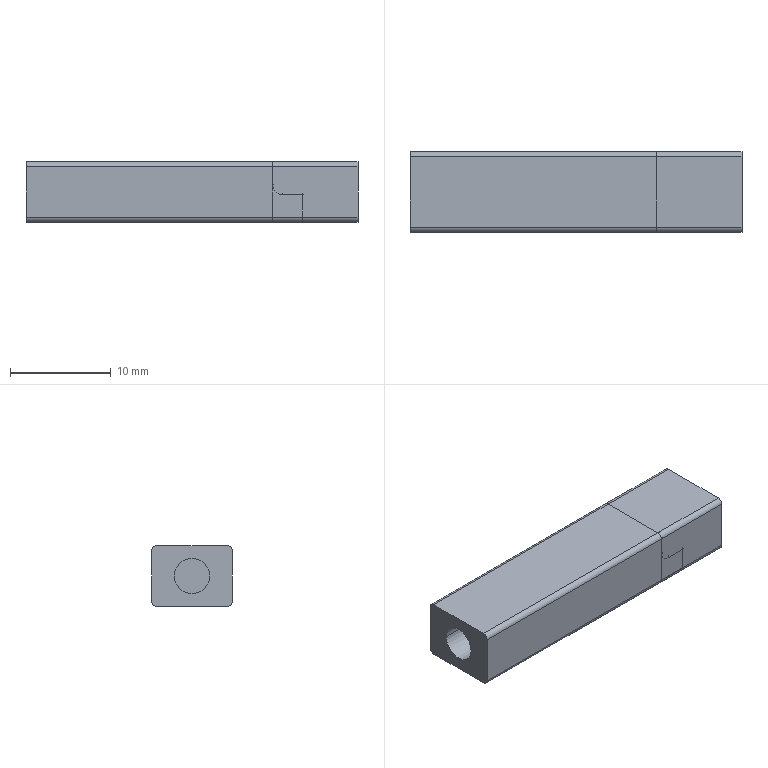NC program | NX | posted with a generic post | part box 33 x 8 x 6 mm
Whole program:
N10 G17 G21 G94 G90
(HOLE_MILLING , TOOL : D2)
N12 T12 M6
N14 G54
N16 G17 G0 G90 X0. Y0. B0. C0. S9500 M3
N18 G43 Z30. H12
N20 Z0.5
N22 G94 G3 X-0.375 Y0.375 R0.375 F1100.
N24 X-0.75 Y0. R0.375
N26 X-0.75 Y0. Z0.4 I0.75 J0.
N28 X-0.75 Y0. Z0.3 I0.75 J0.
N30 X-0.75 Y0. Z0.2 I0.75 J0.
N32 X-0.75 Y0. Z0.1 I0.75 J0.
N34 X-0.75 Y0. Z0. I0.75 J0.
N36 X-0.75 Y0. Z-0.1 I0.75 J0.
N38 X-0.75 Y0. Z-0.2 I0.75 J0.
N40 X-0.75 Y0. Z-0.3 I0.75 J0.
N42 X-0.75 Y0. Z-0.4 I0.75 J0.
N44 X-0.75 Y0. Z-0.5 I0.75 J0.
N46 X-0.75 Y0. Z-0.6 I0.75 J0.
N48 X-0.75 Y0. Z-0.7 I0.75 J0.
N50 X-0.75 Y0. Z-0.8 I0.75 J0.
N52 X-0.75 Y0. Z-0.9 I0.75 J0.
N54 X-0.75 Y0. Z-1. I0.75 J0.
N56 X-0.75 Y0. Z-1.1 I0.75 J0.
N58 X-0.75 Y0. Z-1.2 I0.75 J0.
N60 X-0.75 Y0. Z-1.3 I0.75 J0.
N62 X-0.75 Y0. Z-1.4 I0.75 J0.
N64 X-0.75 Y0. Z-1.5 I0.75 J0.
N66 X-0.75 Y0. Z-1.6 I0.75 J0.
N68 X-0.75 Y0. Z-1.7 I0.75 J0.
N70 X-0.75 Y0. Z-1.8 I0.75 J0.
N72 X-0.75 Y0. Z-1.9 I0.75 J0.
N74 X-0.75 Y0. Z-2. I0.75 J0.
N76 X-0.75 Y0. Z-2.1 I0.75 J0.
N78 X-0.75 Y0. Z-2.2 I0.75 J0.
N80 X-0.75 Y0. Z-2.3 I0.75 J0.
N82 X-0.75 Y0. Z-2.4 I0.75 J0.
N84 X-0.75 Y0. Z-2.5 I0.75 J0.
N86 X-0.75 Y0. Z-2.6 I0.75 J0.
N88 X-0.75 Y0. Z-2.7 I0.75 J0.
N90 X-0.75 Y0. Z-2.8 I0.75 J0.
N92 X-0.75 Y0. Z-2.9 I0.75 J0.
N94 X-0.75 Y0. Z-3. I0.75 J0.
N96 X-0.75 Y0. Z-3.1 I0.75 J0.
N98 X-0.75 Y0. Z-3.2 I0.75 J0.
N100 X-0.75 Y0. Z-3.3 I0.75 J0.
N102 X-0.75 Y0. Z-3.4 I0.75 J0.
N104 X-0.75 Y0. Z-3.5 I0.75 J0.
N106 X-0.75 Y0. Z-3.6 I0.75 J0.
N108 X-0.75 Y0. Z-3.7 I0.75 J0.
N110 X-0.75 Y0. Z-3.8 I0.75 J0.
N112 X-0.75 Y0. Z-3.9 I0.75 J0.
N114 X-0.75 Y0. Z-4. I0.75 J0.
N116 X-0.75 Y0. Z-4.1 I0.75 J0.
N118 X-0.75 Y0. Z-4.2 I0.75 J0.
N120 X-0.75 Y0. Z-4.3 I0.75 J0.
N122 X-0.75 Y0. Z-4.4 I0.75 J0.
N124 X-0.75 Y0. Z-4.5 I0.75 J0.
N126 X-0.75 Y0. Z-4.6 I0.75 J0.
N128 X-0.75 Y0. Z-4.7 I0.75 J0.
N130 X-0.75 Y0. Z-4.8 I0.75 J0.
N132 X-0.75 Y0. Z-4.9 I0.75 J0.
N134 X-0.75 Y0. Z-5. I0.75 J0.
N136 X-0.75 Y0. Z-5.1 I0.75 J0.
N138 X-0.75 Y0. Z-5.2 I0.75 J0.
N140 X-0.75 Y0. Z-5.3 I0.75 J0.
N142 X-0.75 Y0. Z-5.4 I0.75 J0.
N144 X-0.75 Y0. Z-5.5 I0.75 J0.
N146 X-0.75 Y0. Z-5.6 I0.75 J0.
N148 X-0.75 Y0. Z-5.7 I0.75 J0.
N150 X-0.75 Y0. Z-5.8 I0.75 J0.
N152 X-0.75 Y0. Z-5.9 I0.75 J0.
N154 X-0.75 Y0. Z-6. I0.75 J0.
N156 X-0.75 Y0. Z-6.1 I0.75 J0.
N158 X-0.75 Y0. Z-6.2 I0.75 J0.
N160 X-0.75 Y0. Z-6.3 I0.75 J0.
N162 X-0.75 Y0. Z-6.4 I0.75 J0.
N164 X-0.75 Y0. Z-6.5 I0.75 J0.
N166 X-0.75 Y0. Z-6.6 I0.75 J0.
N168 X-0.75 Y0. Z-6.7 I0.75 J0.
N170 X-0.75 Y0. Z-6.8 I0.75 J0.
N172 X-0.75 Y0. Z-6.9 I0.75 J0.
N174 X-0.75 Y0. Z-7. I0.75 J0.
N176 X-0.75 Y0. Z-7.1 I0.75 J0.
N178 X-0.75 Y0. Z-7.2 I0.75 J0.
N180 X-0.75 Y0. Z-7.3 I0.75 J0.
N182 X-0.75 Y0. Z-7.4 I0.75 J0.
N184 X-0.75 Y0. Z-7.5 I0.75 J0.
N186 X-0.75 Y0. Z-7.6 I0.75 J0.
N188 X-0.75 Y0. Z-7.7 I0.75 J0.
N190 X-0.75 Y0. Z-7.8 I0.75 J0.
N192 X-0.75 Y0. Z-7.9 I0.75 J0.
N194 X-0.75 Y0. Z-8. I0.75 J0.
N196 X-0.75 Y0. Z-8.1 I0.75 J0.
N198 X-0.75 Y0. Z-8.2 I0.75 J0.
N200 X-0.75 Y0. Z-8.3 I0.75 J0.
N202 X-0.75 Y0. Z-8.4 I0.75 J0.
N204 X-0.75 Y0. Z-8.5 I0.75 J0.
N206 X-0.75 Y0. Z-8.6 I0.75 J0.
N208 X-0.75 Y0. Z-8.7 I0.75 J0.
N210 X-0.75 Y0. Z-8.8 I0.75 J0.
N212 X-0.75 Y0. Z-8.9 I0.75 J0.
N214 X-0.75 Y0. Z-9. I0.75 J0.
N216 X-0.75 Y0. Z-9.1 I0.75 J0.
N218 X-0.75 Y0. Z-9.2 I0.75 J0.
N220 X-0.75 Y0. Z-9.3 I0.75 J0.
N222 X-0.75 Y0. Z-9.4 I0.75 J0.
N224 X-0.75 Y0. Z-9.5 I0.75 J0.
N226 X-0.75 Y0. Z-9.6 I0.75 J0.
N228 X-0.75 Y0. Z-9.7 I0.75 J0.
N230 X-0.75 Y0. Z-9.8 I0.75 J0.
N232 X-0.75 Y0. Z-9.9 I0.75 J0.
N234 X-0.75 Y0. Z-10. I0.75 J0.
N236 X0. Y-0.75 R0.75
N238 X-0.75 Y0. R-0.75
N240 X-0.375 Y-0.375 R0.375
N242 X0. Y0. R0.375
N244 G0 Z30.
N246 M5
(ZLEVEL_PROFILE_1_COPY_1_COPY , TOOL : D4A45)
N248 T02 M6
N250 G54
N252 G17 G0 G90 X0. Y-0.791 B0. C0. S9500 M3
N254 G43 Z30. H2
N256 Z1.
N258 G94 G1 Z-1. F1000.
N260 G3 X0.791 Y0. R0.791
N262 X0. Y-0.791 R-0.791
N264 X0.346 Y-0.591 R0.4
N266 G1 Z0.
N268 G0 Z30.
N270 X4.139 Y-4.666
N272 Z0.
N274 G1 Z-1.
N276 X3.846 Y-4.159
N278 G3 X3.5 Y-3.959 R0.4
N280 G1 X-3.5
N282 G2 X-4.959 Y-2.5 R1.459
N284 G1 Y2.5
N286 G2 X-3.5 Y3.959 R1.459
N288 G1 X3.5
N290 G2 X4.959 Y2.5 R1.459
N292 G1 Y-2.5
N294 G2 X3.5 Y-3.959 R1.459
N296 G3 X3.154 Y-4.159 R0.4
N298 G1 X2.807 Y-4.759
N300 Z0.
N302 G0 Z30.
N304 M5
N306 M2